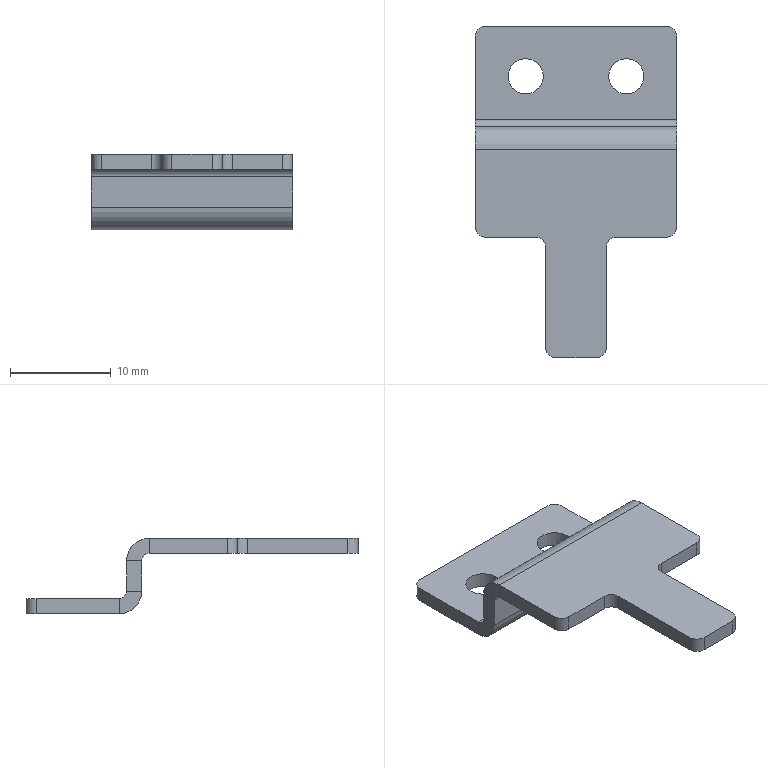Part | STEP file | 10-17 shaft sensor plate (Default) | 1 solid | 38 faces | box 20 x 33 x 7.5 mm | volume 849.566 mm3 | plane 22 | cylinder 16 | commonest cylinder face diameters 2 x8 3.5 x4 1.473 x2 4.473 x2
STEP:
#1=CARTESIAN_POINT('',(-6.75,0.,-1.5));
#2=VERTEX_POINT('',#1);
#3=CARTESIAN_POINT('',(-3.25,0.,-1.5));
#4=VERTEX_POINT('',#3);
#5=CARTESIAN_POINT('',(-5.,0.,-1.5));
#6=DIRECTION('',(0.,0.,1.));
#7=DIRECTION('',(1.,0.,0.));
#8=AXIS2_PLACEMENT_3D('',#5,#6,#7);
#9=CIRCLE('',#8,1.75);
#10=EDGE_CURVE('',#2,#4,#9,.T.);
#11=ORIENTED_EDGE('',*,*,#10,.F.);
#12=CARTESIAN_POINT('',(-6.75,0.,0.));
#13=VERTEX_POINT('',#12);
#14=CARTESIAN_POINT('',(-6.75,0.,0.));
#15=DIRECTION('',(0.,0.,1.));
#16=VECTOR('',#15,1000.);
#17=LINE('',#14,#16);
#18=EDGE_CURVE('',#2,#13,#17,.T.);
#19=ORIENTED_EDGE('',*,*,#18,.T.);
#20=CARTESIAN_POINT('',(-3.25,0.,0.));
#21=VERTEX_POINT('',#20);
#22=CARTESIAN_POINT('',(-5.,0.,0.));
#23=DIRECTION('',(0.,0.,1.));
#24=DIRECTION('',(1.,0.,0.));
#25=AXIS2_PLACEMENT_3D('',#22,#23,#24);
#26=CIRCLE('',#25,1.75);
#27=EDGE_CURVE('',#13,#21,#26,.T.);
#28=ORIENTED_EDGE('',*,*,#27,.T.);
#29=CARTESIAN_POINT('',(-3.25,0.,0.));
#30=DIRECTION('',(0.,0.,1.));
#31=VECTOR('',#30,1000.);
#32=LINE('',#29,#31);
#33=EDGE_CURVE('',#4,#21,#32,.T.);
#34=ORIENTED_EDGE('',*,*,#33,.F.);
#35=EDGE_LOOP('',(#11,#19,#28,#34));
#36=FACE_OUTER_BOUND('',#35,.T.);
#37=CARTESIAN_POINT('',(-5.,0.,0.));
#38=DIRECTION('',(0.,0.,1.));
#39=DIRECTION('',(1.,0.,0.));
#40=AXIS2_PLACEMENT_3D('',#37,#38,#39);
#41=CYLINDRICAL_SURFACE('',#40,1.75);
#42=ADVANCED_FACE('',(#36),#41,.F.);
#43=CARTESIAN_POINT('',(3.25,0.,-1.5));
#44=VERTEX_POINT('',#43);
#45=CARTESIAN_POINT('',(6.75,0.,-1.5));
#46=VERTEX_POINT('',#45);
#47=CARTESIAN_POINT('',(5.,0.,-1.5));
#48=DIRECTION('',(0.,0.,1.));
#49=DIRECTION('',(1.,0.,0.));
#50=AXIS2_PLACEMENT_3D('',#47,#48,#49);
#51=CIRCLE('',#50,1.75);
#52=EDGE_CURVE('',#44,#46,#51,.T.);
#53=ORIENTED_EDGE('',*,*,#52,.F.);
#54=CARTESIAN_POINT('',(3.25,0.,0.));
#55=VERTEX_POINT('',#54);
#56=CARTESIAN_POINT('',(3.25,0.,0.));
#57=DIRECTION('',(0.,0.,1.));
#58=VECTOR('',#57,1000.);
#59=LINE('',#56,#58);
#60=EDGE_CURVE('',#44,#55,#59,.T.);
#61=ORIENTED_EDGE('',*,*,#60,.T.);
#62=CARTESIAN_POINT('',(6.75,0.,0.));
#63=VERTEX_POINT('',#62);
#64=CARTESIAN_POINT('',(5.,0.,0.));
#65=DIRECTION('',(0.,0.,1.));
#66=DIRECTION('',(1.,0.,0.));
#67=AXIS2_PLACEMENT_3D('',#64,#65,#66);
#68=CIRCLE('',#67,1.75);
#69=EDGE_CURVE('',#55,#63,#68,.T.);
#70=ORIENTED_EDGE('',*,*,#69,.T.);
#71=CARTESIAN_POINT('',(6.75,0.,0.));
#72=DIRECTION('',(0.,0.,1.));
#73=VECTOR('',#72,1000.);
#74=LINE('',#71,#73);
#75=EDGE_CURVE('',#46,#63,#74,.T.);
#76=ORIENTED_EDGE('',*,*,#75,.F.);
#77=EDGE_LOOP('',(#53,#61,#70,#76));
#78=FACE_OUTER_BOUND('',#77,.T.);
#79=CARTESIAN_POINT('',(5.,0.,0.));
#80=DIRECTION('',(0.,0.,1.));
#81=DIRECTION('',(1.,0.,0.));
#82=AXIS2_PLACEMENT_3D('',#79,#80,#81);
#83=CYLINDRICAL_SURFACE('',#82,1.75);
#84=ADVANCED_FACE('',(#78),#83,.F.);
#85=CARTESIAN_POINT('',(-10.,-6.5,0.7366));
#86=VERTEX_POINT('',#85);
#87=CARTESIAN_POINT('',(-10.,-6.5,3.763));
#88=VERTEX_POINT('',#87);
#89=CARTESIAN_POINT('',(-10.,-6.5,4.5));
#90=DIRECTION('',(0.,0.,1.));
#91=VECTOR('',#90,1000.);
#92=LINE('',#89,#91);
#93=EDGE_CURVE('',#86,#88,#92,.T.);
#94=ORIENTED_EDGE('',*,*,#93,.T.);
#95=CARTESIAN_POINT('',(-10.,-5.,3.763));
#96=VERTEX_POINT('',#95);
#97=CARTESIAN_POINT('',(-10.,-6.5,3.763));
#98=DIRECTION('',(0.,1.,0.));
#99=VECTOR('',#98,1000.);
#100=LINE('',#97,#99);
#101=EDGE_CURVE('',#88,#96,#100,.T.);
#102=ORIENTED_EDGE('',*,*,#101,.T.);
#103=CARTESIAN_POINT('',(-10.,-5.,0.7366));
#104=VERTEX_POINT('',#103);
#105=CARTESIAN_POINT('',(-10.,-5.,4.5));
#106=DIRECTION('',(0.,0.,1.));
#107=VECTOR('',#106,1000.);
#108=LINE('',#105,#107);
#109=EDGE_CURVE('',#104,#96,#108,.T.);
#110=ORIENTED_EDGE('',*,*,#109,.F.);
#111=CARTESIAN_POINT('',(-10.,-5.,0.7366));
#112=DIRECTION('',(0.,-1.,0.));
#113=VECTOR('',#112,1000.);
#114=LINE('',#111,#113);
#115=EDGE_CURVE('',#104,#86,#114,.T.);
#116=ORIENTED_EDGE('',*,*,#115,.T.);
#117=EDGE_LOOP('',(#94,#102,#110,#116));
#118=FACE_OUTER_BOUND('',#117,.T.);
#119=CARTESIAN_POINT('',(-10.,-6.5,4.5));
#120=DIRECTION('',(-1.,0.,0.));
#121=DIRECTION('',(0.,0.,1.));
#122=AXIS2_PLACEMENT_3D('',#119,#120,#121);
#123=PLANE('',#122);
#124=ADVANCED_FACE('',(#118),#123,.T.);
#125=CARTESIAN_POINT('',(10.,-6.5,3.763));
#126=VERTEX_POINT('',#125);
#127=CARTESIAN_POINT('',(10.,-6.5,0.7366));
#128=VERTEX_POINT('',#127);
#129=CARTESIAN_POINT('',(10.,-6.5,0.));
#130=DIRECTION('',(0.,0.,-1.));
#131=VECTOR('',#130,1000.);
#132=LINE('',#129,#131);
#133=EDGE_CURVE('',#126,#128,#132,.T.);
#134=ORIENTED_EDGE('',*,*,#133,.F.);
#135=CARTESIAN_POINT('',(-10.,-6.5,3.763));
#136=DIRECTION('',(1.,0.,0.));
#137=VECTOR('',#136,1000.);
#138=LINE('',#135,#137);
#139=EDGE_CURVE('',#88,#126,#138,.T.);
#140=ORIENTED_EDGE('',*,*,#139,.F.);
#141=ORIENTED_EDGE('',*,*,#93,.F.);
#142=CARTESIAN_POINT('',(10.,-6.5,0.7366));
#143=DIRECTION('',(1.,0.,0.));
#144=VECTOR('',#143,1000.);
#145=LINE('',#142,#144);
#146=EDGE_CURVE('',#86,#128,#145,.T.);
#147=ORIENTED_EDGE('',*,*,#146,.T.);
#148=EDGE_LOOP('',(#134,#140,#141,#147));
#149=FACE_OUTER_BOUND('',#148,.T.);
#150=CARTESIAN_POINT('',(10.,-6.5,0.));
#151=DIRECTION('',(0.,-1.,0.));
#152=DIRECTION('',(0.,0.,-1.));
#153=AXIS2_PLACEMENT_3D('',#150,#151,#152);
#154=PLANE('',#153);
#155=ADVANCED_FACE('',(#149),#154,.T.);
#156=CARTESIAN_POINT('',(10.,-5.,3.763));
#157=VERTEX_POINT('',#156);
#158=CARTESIAN_POINT('',(-10.,-5.,3.763));
#159=DIRECTION('',(1.,0.,0.));
#160=VECTOR('',#159,1000.);
#161=LINE('',#158,#160);
#162=EDGE_CURVE('',#96,#157,#161,.T.);
#163=ORIENTED_EDGE('',*,*,#162,.T.);
#164=CARTESIAN_POINT('',(10.,-5.,0.7366));
#165=VERTEX_POINT('',#164);
#166=CARTESIAN_POINT('',(10.,-5.,0.));
#167=DIRECTION('',(0.,0.,-1.));
#168=VECTOR('',#167,1000.);
#169=LINE('',#166,#168);
#170=EDGE_CURVE('',#157,#165,#169,.T.);
#171=ORIENTED_EDGE('',*,*,#170,.T.);
#172=CARTESIAN_POINT('',(-10.,-5.,0.7366));
#173=DIRECTION('',(1.,0.,0.));
#174=VECTOR('',#173,1000.);
#175=LINE('',#172,#174);
#176=EDGE_CURVE('',#104,#165,#175,.T.);
#177=ORIENTED_EDGE('',*,*,#176,.F.);
#178=ORIENTED_EDGE('',*,*,#109,.T.);
#179=EDGE_LOOP('',(#163,#171,#177,#178));
#180=FACE_OUTER_BOUND('',#179,.T.);
#181=CARTESIAN_POINT('',(10.,-5.,0.));
#182=DIRECTION('',(0.,-1.,0.));
#183=DIRECTION('',(0.,0.,-1.));
#184=AXIS2_PLACEMENT_3D('',#181,#182,#183);
#185=PLANE('',#184);
#186=ADVANCED_FACE('',(#180),#185,.F.);
#187=CARTESIAN_POINT('',(10.,-4.263,-1.5));
#188=VERTEX_POINT('',#187);
#189=CARTESIAN_POINT('',(10.,4.,-1.5));
#190=VERTEX_POINT('',#189);
#191=CARTESIAN_POINT('',(10.,5.,-1.5));
#192=DIRECTION('',(0.,1.,0.));
#193=VECTOR('',#192,1000.);
#194=LINE('',#191,#193);
#195=EDGE_CURVE('',#188,#190,#194,.T.);
#196=ORIENTED_EDGE('',*,*,#195,.T.);
#197=CARTESIAN_POINT('',(10.,4.,0.));
#198=VERTEX_POINT('',#197);
#199=CARTESIAN_POINT('',(10.,4.,-1.5));
#200=DIRECTION('',(0.,0.,1.));
#201=VECTOR('',#200,1000.);
#202=LINE('',#199,#201);
#203=EDGE_CURVE('',#190,#198,#202,.T.);
#204=ORIENTED_EDGE('',*,*,#203,.T.);
#205=CARTESIAN_POINT('',(10.,-4.263,0.));
#206=VERTEX_POINT('',#205);
#207=CARTESIAN_POINT('',(10.,5.,0.));
#208=DIRECTION('',(0.,1.,0.));
#209=VECTOR('',#208,1000.);
#210=LINE('',#207,#209);
#211=EDGE_CURVE('',#206,#198,#210,.T.);
#212=ORIENTED_EDGE('',*,*,#211,.F.);
#213=CARTESIAN_POINT('',(10.,-4.263,0.));
#214=DIRECTION('',(0.,0.,-1.));
#215=VECTOR('',#214,1000.);
#216=LINE('',#213,#215);
#217=EDGE_CURVE('',#206,#188,#216,.T.);
#218=ORIENTED_EDGE('',*,*,#217,.T.);
#219=EDGE_LOOP('',(#196,#204,#212,#218));
#220=FACE_OUTER_BOUND('',#219,.T.);
#221=CARTESIAN_POINT('',(10.,5.,-1.5));
#222=DIRECTION('',(1.,0.,0.));
#223=DIRECTION('',(0.,1.,0.));
#224=AXIS2_PLACEMENT_3D('',#221,#222,#223);
#225=PLANE('',#224);
#226=ADVANCED_FACE('',(#220),#225,.T.);
#227=CARTESIAN_POINT('',(5.,0.,-1.5));
#228=DIRECTION('',(0.,0.,1.));
#229=DIRECTION('',(1.,0.,0.));
#230=AXIS2_PLACEMENT_3D('',#227,#228,#229);
#231=CIRCLE('',#230,1.75);
#232=EDGE_CURVE('',#46,#44,#231,.T.);
#233=ORIENTED_EDGE('',*,*,#232,.T.);
#234=ORIENTED_EDGE('',*,*,#52,.T.);
#235=EDGE_LOOP('',(#233,#234));
#236=FACE_BOUND('',#235,.T.);
#237=CARTESIAN_POINT('',(-5.,0.,-1.5));
#238=DIRECTION('',(0.,0.,1.));
#239=DIRECTION('',(1.,0.,0.));
#240=AXIS2_PLACEMENT_3D('',#237,#238,#239);
#241=CIRCLE('',#240,1.75);
#242=EDGE_CURVE('',#4,#2,#241,.T.);
#243=ORIENTED_EDGE('',*,*,#242,.T.);
#244=ORIENTED_EDGE('',*,*,#10,.T.);
#245=EDGE_LOOP('',(#243,#244));
#246=FACE_BOUND('',#245,.T.);
#247=CARTESIAN_POINT('',(-10.,4.,-1.5));
#248=VERTEX_POINT('',#247);
#249=CARTESIAN_POINT('',(-10.,-4.263,-1.5));
#250=VERTEX_POINT('',#249);
#251=CARTESIAN_POINT('',(-10.,5.,-1.5));
#252=DIRECTION('',(0.,-1.,0.));
#253=VECTOR('',#252,1000.);
#254=LINE('',#251,#253);
#255=EDGE_CURVE('',#248,#250,#254,.T.);
#256=ORIENTED_EDGE('',*,*,#255,.F.);
#257=CARTESIAN_POINT('',(-9.,5.,-1.5));
#258=VERTEX_POINT('',#257);
#259=CARTESIAN_POINT('',(-9.,4.,-1.5));
#260=DIRECTION('',(0.,0.,-1.));
#261=DIRECTION('',(1.,0.,0.));
#262=AXIS2_PLACEMENT_3D('',#259,#260,#261);
#263=CIRCLE('',#262,1.);
#264=EDGE_CURVE('',#248,#258,#263,.T.);
#265=ORIENTED_EDGE('',*,*,#264,.T.);
#266=CARTESIAN_POINT('',(9.,5.,-1.5));
#267=VERTEX_POINT('',#266);
#268=CARTESIAN_POINT('',(-10.,5.,-1.5));
#269=DIRECTION('',(-1.,0.,0.));
#270=VECTOR('',#269,1000.);
#271=LINE('',#268,#270);
#272=EDGE_CURVE('',#267,#258,#271,.T.);
#273=ORIENTED_EDGE('',*,*,#272,.F.);
#274=CARTESIAN_POINT('',(9.,4.,-1.5));
#275=DIRECTION('',(0.,0.,-1.));
#276=DIRECTION('',(1.,0.,0.));
#277=AXIS2_PLACEMENT_3D('',#274,#275,#276);
#278=CIRCLE('',#277,1.);
#279=EDGE_CURVE('',#267,#190,#278,.T.);
#280=ORIENTED_EDGE('',*,*,#279,.T.);
#281=ORIENTED_EDGE('',*,*,#195,.F.);
#282=CARTESIAN_POINT('',(10.,-4.263,-1.5));
#283=DIRECTION('',(-1.,0.,0.));
#284=VECTOR('',#283,1000.);
#285=LINE('',#282,#284);
#286=EDGE_CURVE('',#188,#250,#285,.T.);
#287=ORIENTED_EDGE('',*,*,#286,.T.);
#288=EDGE_LOOP('',(#256,#265,#273,#280,#281,#287));
#289=FACE_OUTER_BOUND('',#288,.T.);
#290=CARTESIAN_POINT('',(10.,-5.,-1.5));
#291=DIRECTION('',(0.,0.,1.));
#292=DIRECTION('',(1.,0.,0.));
#293=AXIS2_PLACEMENT_3D('',#290,#291,#292);
#294=PLANE('',#293);
#295=ADVANCED_FACE('',(#236,#246,#289),#294,.F.);
#296=CARTESIAN_POINT('',(5.,0.,0.));
#297=DIRECTION('',(0.,0.,1.));
#298=DIRECTION('',(1.,0.,0.));
#299=AXIS2_PLACEMENT_3D('',#296,#297,#298);
#300=CIRCLE('',#299,1.75);
#301=EDGE_CURVE('',#63,#55,#300,.T.);
#302=ORIENTED_EDGE('',*,*,#301,.F.);
#303=ORIENTED_EDGE('',*,*,#69,.F.);
#304=EDGE_LOOP('',(#302,#303));
#305=FACE_BOUND('',#304,.T.);
#306=CARTESIAN_POINT('',(-5.,0.,0.));
#307=DIRECTION('',(0.,0.,1.));
#308=DIRECTION('',(1.,0.,0.));
#309=AXIS2_PLACEMENT_3D('',#306,#307,#308);
#310=CIRCLE('',#309,1.75);
#311=EDGE_CURVE('',#21,#13,#310,.T.);
#312=ORIENTED_EDGE('',*,*,#311,.F.);
#313=ORIENTED_EDGE('',*,*,#27,.F.);
#314=EDGE_LOOP('',(#312,#313));
#315=FACE_BOUND('',#314,.T.);
#316=CARTESIAN_POINT('',(9.,5.,0.));
#317=VERTEX_POINT('',#316);
#318=CARTESIAN_POINT('',(-9.,5.,0.));
#319=VERTEX_POINT('',#318);
#320=CARTESIAN_POINT('',(-10.,5.,0.));
#321=DIRECTION('',(-1.,0.,0.));
#322=VECTOR('',#321,1000.);
#323=LINE('',#320,#322);
#324=EDGE_CURVE('',#317,#319,#323,.T.);
#325=ORIENTED_EDGE('',*,*,#324,.T.);
#326=CARTESIAN_POINT('',(-10.,4.,0.));
#327=VERTEX_POINT('',#326);
#328=CARTESIAN_POINT('',(-9.,4.,0.));
#329=DIRECTION('',(0.,0.,1.));
#330=DIRECTION('',(1.,0.,0.));
#331=AXIS2_PLACEMENT_3D('',#328,#329,#330);
#332=CIRCLE('',#331,1.);
#333=EDGE_CURVE('',#319,#327,#332,.T.);
#334=ORIENTED_EDGE('',*,*,#333,.T.);
#335=CARTESIAN_POINT('',(-10.,-4.263,0.));
#336=VERTEX_POINT('',#335);
#337=CARTESIAN_POINT('',(-10.,5.,0.));
#338=DIRECTION('',(0.,-1.,0.));
#339=VECTOR('',#338,1000.);
#340=LINE('',#337,#339);
#341=EDGE_CURVE('',#327,#336,#340,.T.);
#342=ORIENTED_EDGE('',*,*,#341,.T.);
#343=CARTESIAN_POINT('',(10.,-4.263,0.));
#344=DIRECTION('',(-1.,0.,0.));
#345=VECTOR('',#344,1000.);
#346=LINE('',#343,#345);
#347=EDGE_CURVE('',#206,#336,#346,.T.);
#348=ORIENTED_EDGE('',*,*,#347,.F.);
#349=ORIENTED_EDGE('',*,*,#211,.T.);
#350=CARTESIAN_POINT('',(9.,4.,0.));
#351=DIRECTION('',(0.,0.,1.));
#352=DIRECTION('',(1.,0.,0.));
#353=AXIS2_PLACEMENT_3D('',#350,#351,#352);
#354=CIRCLE('',#353,1.);
#355=EDGE_CURVE('',#198,#317,#354,.T.);
#356=ORIENTED_EDGE('',*,*,#355,.T.);
#357=EDGE_LOOP('',(#325,#334,#342,#348,#349,#356));
#358=FACE_OUTER_BOUND('',#357,.T.);
#359=CARTESIAN_POINT('',(10.,-5.,0.));
#360=DIRECTION('',(0.,0.,1.));
#361=DIRECTION('',(1.,0.,0.));
#362=AXIS2_PLACEMENT_3D('',#359,#360,#361);
#363=PLANE('',#362);
#364=ADVANCED_FACE('',(#305,#315,#358),#363,.T.);
#365=ORIENTED_EDGE('',*,*,#341,.F.);
#366=CARTESIAN_POINT('',(-10.,4.,-1.5));
#367=DIRECTION('',(0.,0.,-1.));
#368=VECTOR('',#367,1000.);
#369=LINE('',#366,#368);
#370=EDGE_CURVE('',#327,#248,#369,.T.);
#371=ORIENTED_EDGE('',*,*,#370,.T.);
#372=ORIENTED_EDGE('',*,*,#255,.T.);
#373=CARTESIAN_POINT('',(-10.,-4.263,0.));
#374=DIRECTION('',(0.,0.,-1.));
#375=VECTOR('',#374,1000.);
#376=LINE('',#373,#375);
#377=EDGE_CURVE('',#336,#250,#376,.T.);
#378=ORIENTED_EDGE('',*,*,#377,.F.);
#379=EDGE_LOOP('',(#365,#371,#372,#378));
#380=FACE_OUTER_BOUND('',#379,.T.);
#381=CARTESIAN_POINT('',(-10.,5.,-1.5));
#382=DIRECTION('',(-1.,0.,0.));
#383=DIRECTION('',(0.,-1.,0.));
#384=AXIS2_PLACEMENT_3D('',#381,#382,#383);
#385=PLANE('',#384);
#386=ADVANCED_FACE('',(#380),#385,.T.);
#387=ORIENTED_EDGE('',*,*,#272,.T.);
#388=CARTESIAN_POINT('',(-9.,5.,-1.5));
#389=DIRECTION('',(0.,0.,1.));
#390=VECTOR('',#389,1000.);
#391=LINE('',#388,#390);
#392=EDGE_CURVE('',#258,#319,#391,.T.);
#393=ORIENTED_EDGE('',*,*,#392,.T.);
#394=ORIENTED_EDGE('',*,*,#324,.F.);
#395=CARTESIAN_POINT('',(9.,5.,-1.5));
#396=DIRECTION('',(0.,0.,-1.));
#397=VECTOR('',#396,1000.);
#398=LINE('',#395,#397);
#399=EDGE_CURVE('',#317,#267,#398,.T.);
#400=ORIENTED_EDGE('',*,*,#399,.T.);
#401=EDGE_LOOP('',(#387,#393,#394,#400));
#402=FACE_OUTER_BOUND('',#401,.T.);
#403=CARTESIAN_POINT('',(-10.,5.,-1.5));
#404=DIRECTION('',(0.,1.,0.));
#405=DIRECTION('',(0.,0.,1.));
#406=AXIS2_PLACEMENT_3D('',#403,#404,#405);
#407=PLANE('',#406);
#408=ADVANCED_FACE('',(#402),#407,.T.);
#409=ORIENTED_EDGE('',*,*,#60,.F.);
#410=ORIENTED_EDGE('',*,*,#232,.F.);
#411=ORIENTED_EDGE('',*,*,#75,.T.);
#412=ORIENTED_EDGE('',*,*,#301,.T.);
#413=EDGE_LOOP('',(#409,#410,#411,#412));
#414=FACE_OUTER_BOUND('',#413,.T.);
#415=CARTESIAN_POINT('',(5.,0.,0.));
#416=DIRECTION('',(0.,0.,1.));
#417=DIRECTION('',(1.,0.,0.));
#418=AXIS2_PLACEMENT_3D('',#415,#416,#417);
#419=CYLINDRICAL_SURFACE('',#418,1.75);
#420=ADVANCED_FACE('',(#414),#419,.F.);
#421=ORIENTED_EDGE('',*,*,#18,.F.);
#422=ORIENTED_EDGE('',*,*,#242,.F.);
#423=ORIENTED_EDGE('',*,*,#33,.T.);
#424=ORIENTED_EDGE('',*,*,#311,.T.);
#425=EDGE_LOOP('',(#421,#422,#423,#424));
#426=FACE_OUTER_BOUND('',#425,.T.);
#427=CARTESIAN_POINT('',(-5.,0.,0.));
#428=DIRECTION('',(0.,0.,1.));
#429=DIRECTION('',(1.,0.,0.));
#430=AXIS2_PLACEMENT_3D('',#427,#428,#429);
#431=CYLINDRICAL_SURFACE('',#430,1.75);
#432=ADVANCED_FACE('',(#426),#431,.F.);
#433=ORIENTED_EDGE('',*,*,#115,.F.);
#434=CARTESIAN_POINT('',(-10.,-4.263,0.7366));
#435=DIRECTION('',(-1.,0.,0.));
#436=DIRECTION('',(0.,0.,-1.));
#437=AXIS2_PLACEMENT_3D('',#434,#435,#436);
#438=CIRCLE('',#437,0.7366);
#439=EDGE_CURVE('',#336,#104,#438,.T.);
#440=ORIENTED_EDGE('',*,*,#439,.F.);
#441=ORIENTED_EDGE('',*,*,#377,.T.);
#442=CARTESIAN_POINT('',(-10.,-4.263,0.7366));
#443=DIRECTION('',(-1.,0.,0.));
#444=DIRECTION('',(0.,0.,-1.));
#445=AXIS2_PLACEMENT_3D('',#442,#443,#444);
#446=CIRCLE('',#445,2.237);
#447=EDGE_CURVE('',#250,#86,#446,.T.);
#448=ORIENTED_EDGE('',*,*,#447,.T.);
#449=EDGE_LOOP('',(#433,#440,#441,#448));
#450=FACE_OUTER_BOUND('',#449,.T.);
#451=CARTESIAN_POINT('',(-10.,-4.263,0.7366));
#452=DIRECTION('',(-1.,0.,0.));
#453=DIRECTION('',(0.,0.,1.));
#454=AXIS2_PLACEMENT_3D('',#451,#452,#453);
#455=PLANE('',#454);
#456=ADVANCED_FACE('',(#450),#455,.T.);
#457=CARTESIAN_POINT('',(10.,-4.263,0.7366));
#458=DIRECTION('',(1.,0.,0.));
#459=DIRECTION('',(0.,0.,-1.));
#460=AXIS2_PLACEMENT_3D('',#457,#458,#459);
#461=CIRCLE('',#460,0.7366);
#462=EDGE_CURVE('',#165,#206,#461,.T.);
#463=ORIENTED_EDGE('',*,*,#462,.F.);
#464=CARTESIAN_POINT('',(10.,-5.,0.7366));
#465=DIRECTION('',(0.,-1.,0.));
#466=VECTOR('',#465,1000.);
#467=LINE('',#464,#466);
#468=EDGE_CURVE('',#165,#128,#467,.T.);
#469=ORIENTED_EDGE('',*,*,#468,.T.);
#470=CARTESIAN_POINT('',(10.,-4.263,0.7366));
#471=DIRECTION('',(1.,0.,0.));
#472=DIRECTION('',(0.,0.,-1.));
#473=AXIS2_PLACEMENT_3D('',#470,#471,#472);
#474=CIRCLE('',#473,2.237);
#475=EDGE_CURVE('',#128,#188,#474,.T.);
#476=ORIENTED_EDGE('',*,*,#475,.T.);
#477=ORIENTED_EDGE('',*,*,#217,.F.);
#478=EDGE_LOOP('',(#463,#469,#476,#477));
#479=FACE_OUTER_BOUND('',#478,.T.);
#480=CARTESIAN_POINT('',(10.,-4.263,0.7366));
#481=DIRECTION('',(-1.,0.,0.));
#482=DIRECTION('',(0.,0.,1.));
#483=AXIS2_PLACEMENT_3D('',#480,#481,#482);
#484=PLANE('',#483);
#485=ADVANCED_FACE('',(#479),#484,.F.);
#486=ORIENTED_EDGE('',*,*,#286,.F.);
#487=ORIENTED_EDGE('',*,*,#475,.F.);
#488=ORIENTED_EDGE('',*,*,#146,.F.);
#489=ORIENTED_EDGE('',*,*,#447,.F.);
#490=EDGE_LOOP('',(#486,#487,#488,#489));
#491=FACE_OUTER_BOUND('',#490,.T.);
#492=CARTESIAN_POINT('',(10.,-4.263,0.7366));
#493=DIRECTION('',(1.,0.,0.));
#494=DIRECTION('',(0.,-1.,0.));
#495=AXIS2_PLACEMENT_3D('',#492,#493,#494);
#496=CYLINDRICAL_SURFACE('',#495,2.237);
#497=ADVANCED_FACE('',(#491),#496,.T.);
#498=ORIENTED_EDGE('',*,*,#347,.T.);
#499=ORIENTED_EDGE('',*,*,#439,.T.);
#500=ORIENTED_EDGE('',*,*,#176,.T.);
#501=ORIENTED_EDGE('',*,*,#462,.T.);
#502=EDGE_LOOP('',(#498,#499,#500,#501));
#503=FACE_OUTER_BOUND('',#502,.T.);
#504=CARTESIAN_POINT('',(10.,-4.263,0.7366));
#505=DIRECTION('',(1.,0.,0.));
#506=DIRECTION('',(0.,-1.,0.));
#507=AXIS2_PLACEMENT_3D('',#504,#505,#506);
#508=CYLINDRICAL_SURFACE('',#507,0.7366);
#509=ADVANCED_FACE('',(#503),#508,.F.);
#510=CARTESIAN_POINT('',(10.,-6.5,3.763));
#511=DIRECTION('',(0.,1.,0.));
#512=VECTOR('',#511,1000.);
#513=LINE('',#510,#512);
#514=EDGE_CURVE('',#126,#157,#513,.T.);
#515=ORIENTED_EDGE('',*,*,#514,.F.);
#516=ORIENTED_EDGE('',*,*,#133,.T.);
#517=ORIENTED_EDGE('',*,*,#468,.F.);
#518=ORIENTED_EDGE('',*,*,#170,.F.);
#519=EDGE_LOOP('',(#515,#516,#517,#518));
#520=FACE_OUTER_BOUND('',#519,.T.);
#521=CARTESIAN_POINT('',(10.,-6.5,0.));
#522=DIRECTION('',(1.,0.,0.));
#523=DIRECTION('',(0.,0.,-1.));
#524=AXIS2_PLACEMENT_3D('',#521,#522,#523);
#525=PLANE('',#524);
#526=ADVANCED_FACE('',(#520),#525,.T.);
#527=CARTESIAN_POINT('',(10.,-7.237,4.5));
#528=VERTEX_POINT('',#527);
#529=CARTESIAN_POINT('',(10.,-7.237,6.));
#530=VERTEX_POINT('',#529);
#531=CARTESIAN_POINT('',(10.,-7.237,4.5));
#532=DIRECTION('',(0.,0.,1.));
#533=VECTOR('',#532,1000.);
#534=LINE('',#531,#533);
#535=EDGE_CURVE('',#528,#530,#534,.T.);
#536=ORIENTED_EDGE('',*,*,#535,.F.);
#537=CARTESIAN_POINT('',(10.,-7.237,3.763));
#538=DIRECTION('',(1.,0.,0.));
#539=DIRECTION('',(0.,0.,1.));
#540=AXIS2_PLACEMENT_3D('',#537,#538,#539);
#541=CIRCLE('',#540,0.7366);
#542=EDGE_CURVE('',#126,#528,#541,.T.);
#543=ORIENTED_EDGE('',*,*,#542,.F.);
#544=ORIENTED_EDGE('',*,*,#514,.T.);
#545=CARTESIAN_POINT('',(10.,-7.237,3.763));
#546=DIRECTION('',(1.,0.,0.));
#547=DIRECTION('',(0.,0.,1.));
#548=AXIS2_PLACEMENT_3D('',#545,#546,#547);
#549=CIRCLE('',#548,2.237);
#550=EDGE_CURVE('',#157,#530,#549,.T.);
#551=ORIENTED_EDGE('',*,*,#550,.T.);
#552=EDGE_LOOP('',(#536,#543,#544,#551));
#553=FACE_OUTER_BOUND('',#552,.T.);
#554=CARTESIAN_POINT('',(10.,-7.237,3.763));
#555=DIRECTION('',(1.,0.,0.));
#556=DIRECTION('',(0.,0.,-1.));
#557=AXIS2_PLACEMENT_3D('',#554,#555,#556);
#558=PLANE('',#557);
#559=ADVANCED_FACE('',(#553),#558,.T.);
#560=CARTESIAN_POINT('',(-10.,-7.237,4.5));
#561=VERTEX_POINT('',#560);
#562=CARTESIAN_POINT('',(-10.,-7.237,3.763));
#563=DIRECTION('',(-1.,0.,0.));
#564=DIRECTION('',(0.,0.,1.));
#565=AXIS2_PLACEMENT_3D('',#562,#563,#564);
#566=CIRCLE('',#565,0.7366);
#567=EDGE_CURVE('',#561,#88,#566,.T.);
#568=ORIENTED_EDGE('',*,*,#567,.F.);
#569=CARTESIAN_POINT('',(-10.,-7.237,6.));
#570=VERTEX_POINT('',#569);
#571=CARTESIAN_POINT('',(-10.,-7.237,4.5));
#572=DIRECTION('',(0.,0.,1.));
#573=VECTOR('',#572,1000.);
#574=LINE('',#571,#573);
#575=EDGE_CURVE('',#561,#570,#574,.T.);
#576=ORIENTED_EDGE('',*,*,#575,.T.);
#577=CARTESIAN_POINT('',(-10.,-7.237,3.763));
#578=DIRECTION('',(-1.,0.,0.));
#579=DIRECTION('',(0.,0.,1.));
#580=AXIS2_PLACEMENT_3D('',#577,#578,#579);
#581=CIRCLE('',#580,2.237);
#582=EDGE_CURVE('',#570,#96,#581,.T.);
#583=ORIENTED_EDGE('',*,*,#582,.T.);
#584=ORIENTED_EDGE('',*,*,#101,.F.);
#585=EDGE_LOOP('',(#568,#576,#583,#584));
#586=FACE_OUTER_BOUND('',#585,.T.);
#587=CARTESIAN_POINT('',(-10.,-7.237,3.763));
#588=DIRECTION('',(1.,0.,0.));
#589=DIRECTION('',(0.,0.,-1.));
#590=AXIS2_PLACEMENT_3D('',#587,#588,#589);
#591=PLANE('',#590);
#592=ADVANCED_FACE('',(#586),#591,.F.);
#593=ORIENTED_EDGE('',*,*,#162,.F.);
#594=ORIENTED_EDGE('',*,*,#582,.F.);
#595=CARTESIAN_POINT('',(-10.,-7.237,6.));
#596=DIRECTION('',(-1.,0.,0.));
#597=VECTOR('',#596,1000.);
#598=LINE('',#595,#597);
#599=EDGE_CURVE('',#530,#570,#598,.T.);
#600=ORIENTED_EDGE('',*,*,#599,.F.);
#601=ORIENTED_EDGE('',*,*,#550,.F.);
#602=EDGE_LOOP('',(#593,#594,#600,#601));
#603=FACE_OUTER_BOUND('',#602,.T.);
#604=CARTESIAN_POINT('',(-10.,-7.237,3.763));
#605=DIRECTION('',(-1.,0.,0.));
#606=DIRECTION('',(0.,0.,1.));
#607=AXIS2_PLACEMENT_3D('',#604,#605,#606);
#608=CYLINDRICAL_SURFACE('',#607,2.237);
#609=ADVANCED_FACE('',(#603),#608,.T.);
#610=ORIENTED_EDGE('',*,*,#139,.T.);
#611=ORIENTED_EDGE('',*,*,#542,.T.);
#612=CARTESIAN_POINT('',(10.,-7.237,4.5));
#613=DIRECTION('',(-1.,0.,0.));
#614=VECTOR('',#613,1000.);
#615=LINE('',#612,#614);
#616=EDGE_CURVE('',#528,#561,#615,.T.);
#617=ORIENTED_EDGE('',*,*,#616,.T.);
#618=ORIENTED_EDGE('',*,*,#567,.T.);
#619=EDGE_LOOP('',(#610,#611,#617,#618));
#620=FACE_OUTER_BOUND('',#619,.T.);
#621=CARTESIAN_POINT('',(-10.,-7.237,3.763));
#622=DIRECTION('',(-1.,0.,0.));
#623=DIRECTION('',(0.,0.,1.));
#624=AXIS2_PLACEMENT_3D('',#621,#622,#623);
#625=CYLINDRICAL_SURFACE('',#624,0.7366);
#626=ADVANCED_FACE('',(#620),#625,.F.);
#627=CARTESIAN_POINT('',(-10.,-15.,4.5));
#628=VERTEX_POINT('',#627);
#629=CARTESIAN_POINT('',(-10.,-6.5,4.5));
#630=DIRECTION('',(0.,1.,0.));
#631=VECTOR('',#630,1000.);
#632=LINE('',#629,#631);
#633=EDGE_CURVE('',#628,#561,#632,.T.);
#634=ORIENTED_EDGE('',*,*,#633,.F.);
#635=CARTESIAN_POINT('',(-10.,-15.,6.));
#636=VERTEX_POINT('',#635);
#637=CARTESIAN_POINT('',(-10.,-15.,6.));
#638=DIRECTION('',(0.,0.,1.));
#639=VECTOR('',#638,1000.);
#640=LINE('',#637,#639);
#641=EDGE_CURVE('',#628,#636,#640,.T.);
#642=ORIENTED_EDGE('',*,*,#641,.T.);
#643=CARTESIAN_POINT('',(-10.,-6.5,6.));
#644=DIRECTION('',(0.,1.,0.));
#645=VECTOR('',#644,1000.);
#646=LINE('',#643,#645);
#647=EDGE_CURVE('',#636,#570,#646,.T.);
#648=ORIENTED_EDGE('',*,*,#647,.T.);
#649=ORIENTED_EDGE('',*,*,#575,.F.);
#650=EDGE_LOOP('',(#634,#642,#648,#649));
#651=FACE_OUTER_BOUND('',#650,.T.);
#652=CARTESIAN_POINT('',(-10.,-6.5,6.));
#653=DIRECTION('',(-1.,0.,0.));
#654=DIRECTION('',(0.,0.,1.));
#655=AXIS2_PLACEMENT_3D('',#652,#653,#654);
#656=PLANE('',#655);
#657=ADVANCED_FACE('',(#651),#656,.T.);
#658=CARTESIAN_POINT('',(10.,-15.,6.));
#659=VERTEX_POINT('',#658);
#660=CARTESIAN_POINT('',(10.,-28.,6.));
#661=DIRECTION('',(0.,-1.,0.));
#662=VECTOR('',#661,1000.);
#663=LINE('',#660,#662);
#664=EDGE_CURVE('',#530,#659,#663,.T.);
#665=ORIENTED_EDGE('',*,*,#664,.T.);
#666=CARTESIAN_POINT('',(10.,-15.,4.5));
#667=VERTEX_POINT('',#666);
#668=CARTESIAN_POINT('',(10.,-15.,4.5));
#669=DIRECTION('',(0.,0.,-1.));
#670=VECTOR('',#669,1000.);
#671=LINE('',#668,#670);
#672=EDGE_CURVE('',#659,#667,#671,.T.);
#673=ORIENTED_EDGE('',*,*,#672,.T.);
#674=CARTESIAN_POINT('',(10.,-28.,4.5));
#675=DIRECTION('',(0.,-1.,0.));
#676=VECTOR('',#675,1000.);
#677=LINE('',#674,#676);
#678=EDGE_CURVE('',#528,#667,#677,.T.);
#679=ORIENTED_EDGE('',*,*,#678,.F.);
#680=ORIENTED_EDGE('',*,*,#535,.T.);
#681=EDGE_LOOP('',(#665,#673,#679,#680));
#682=FACE_OUTER_BOUND('',#681,.T.);
#683=CARTESIAN_POINT('',(10.,-28.,6.));
#684=DIRECTION('',(1.,0.,0.));
#685=DIRECTION('',(0.,0.,-1.));
#686=AXIS2_PLACEMENT_3D('',#683,#684,#685);
#687=PLANE('',#686);
#688=ADVANCED_FACE('',(#682),#687,.T.);
#689=ORIENTED_EDGE('',*,*,#647,.F.);
#690=CARTESIAN_POINT('',(-9.,-16.,6.));
#691=VERTEX_POINT('',#690);
#692=CARTESIAN_POINT('',(-9.,-15.,6.));
#693=DIRECTION('',(0.,0.,1.));
#694=DIRECTION('',(0.,-1.,0.));
#695=AXIS2_PLACEMENT_3D('',#692,#693,#694);
#696=CIRCLE('',#695,1.);
#697=EDGE_CURVE('',#636,#691,#696,.T.);
#698=ORIENTED_EDGE('',*,*,#697,.T.);
#699=CARTESIAN_POINT('',(-4.,-16.,6.));
#700=VERTEX_POINT('',#699);
#701=CARTESIAN_POINT('',(-10.,-16.,6.));
#702=DIRECTION('',(-1.,0.,0.));
#703=VECTOR('',#702,1000.);
#704=LINE('',#701,#703);
#705=EDGE_CURVE('',#700,#691,#704,.T.);
#706=ORIENTED_EDGE('',*,*,#705,.F.);
#707=CARTESIAN_POINT('',(-3.,-17.,6.));
#708=VERTEX_POINT('',#707);
#709=CARTESIAN_POINT('',(-4.,-17.,6.));
#710=DIRECTION('',(0.,0.,-1.));
#711=DIRECTION('',(0.,-1.,0.));
#712=AXIS2_PLACEMENT_3D('',#709,#710,#711);
#713=CIRCLE('',#712,1.);
#714=EDGE_CURVE('',#700,#708,#713,.T.);
#715=ORIENTED_EDGE('',*,*,#714,.T.);
#716=CARTESIAN_POINT('',(-3.,-27.,6.));
#717=VERTEX_POINT('',#716);
#718=CARTESIAN_POINT('',(-3.,-28.,6.));
#719=DIRECTION('',(0.,1.,0.));
#720=VECTOR('',#719,1000.);
#721=LINE('',#718,#720);
#722=EDGE_CURVE('',#717,#708,#721,.T.);
#723=ORIENTED_EDGE('',*,*,#722,.F.);
#724=CARTESIAN_POINT('',(-2.,-28.,6.));
#725=VERTEX_POINT('',#724);
#726=CARTESIAN_POINT('',(-2.,-27.,6.));
#727=DIRECTION('',(0.,0.,1.));
#728=DIRECTION('',(0.,-1.,0.));
#729=AXIS2_PLACEMENT_3D('',#726,#727,#728);
#730=CIRCLE('',#729,1.);
#731=EDGE_CURVE('',#717,#725,#730,.T.);
#732=ORIENTED_EDGE('',*,*,#731,.T.);
#733=CARTESIAN_POINT('',(2.,-28.,6.));
#734=VERTEX_POINT('',#733);
#735=CARTESIAN_POINT('',(-10.,-28.,6.));
#736=DIRECTION('',(-1.,0.,0.));
#737=VECTOR('',#736,1000.);
#738=LINE('',#735,#737);
#739=EDGE_CURVE('',#734,#725,#738,.T.);
#740=ORIENTED_EDGE('',*,*,#739,.F.);
#741=CARTESIAN_POINT('',(3.,-27.,6.));
#742=VERTEX_POINT('',#741);
#743=CARTESIAN_POINT('',(2.,-27.,6.));
#744=DIRECTION('',(0.,0.,1.));
#745=DIRECTION('',(0.,-1.,0.));
#746=AXIS2_PLACEMENT_3D('',#743,#744,#745);
#747=CIRCLE('',#746,1.);
#748=EDGE_CURVE('',#734,#742,#747,.T.);
#749=ORIENTED_EDGE('',*,*,#748,.T.);
#750=CARTESIAN_POINT('',(3.,-17.,6.));
#751=VERTEX_POINT('',#750);
#752=CARTESIAN_POINT('',(3.,-28.,6.));
#753=DIRECTION('',(0.,-1.,0.));
#754=VECTOR('',#753,1000.);
#755=LINE('',#752,#754);
#756=EDGE_CURVE('',#751,#742,#755,.T.);
#757=ORIENTED_EDGE('',*,*,#756,.F.);
#758=CARTESIAN_POINT('',(4.,-16.,6.));
#759=VERTEX_POINT('',#758);
#760=CARTESIAN_POINT('',(4.,-17.,6.));
#761=DIRECTION('',(0.,0.,-1.));
#762=DIRECTION('',(0.,-1.,0.));
#763=AXIS2_PLACEMENT_3D('',#760,#761,#762);
#764=CIRCLE('',#763,1.);
#765=EDGE_CURVE('',#751,#759,#764,.T.);
#766=ORIENTED_EDGE('',*,*,#765,.T.);
#767=CARTESIAN_POINT('',(9.,-16.,6.));
#768=VERTEX_POINT('',#767);
#769=CARTESIAN_POINT('',(10.,-16.,6.));
#770=DIRECTION('',(-1.,0.,0.));
#771=VECTOR('',#770,1000.);
#772=LINE('',#769,#771);
#773=EDGE_CURVE('',#768,#759,#772,.T.);
#774=ORIENTED_EDGE('',*,*,#773,.F.);
#775=CARTESIAN_POINT('',(9.,-15.,6.));
#776=DIRECTION('',(0.,0.,1.));
#777=DIRECTION('',(0.,-1.,0.));
#778=AXIS2_PLACEMENT_3D('',#775,#776,#777);
#779=CIRCLE('',#778,1.);
#780=EDGE_CURVE('',#768,#659,#779,.T.);
#781=ORIENTED_EDGE('',*,*,#780,.T.);
#782=ORIENTED_EDGE('',*,*,#664,.F.);
#783=ORIENTED_EDGE('',*,*,#599,.T.);
#784=EDGE_LOOP('',(#689,#698,#706,#715,#723,#732,#740,#749,#757,#766,#774,#781,#782,#783));
#785=FACE_OUTER_BOUND('',#784,.T.);
#786=CARTESIAN_POINT('',(-10.,-6.5,6.));
#787=DIRECTION('',(0.,0.,1.));
#788=DIRECTION('',(0.,-1.,0.));
#789=AXIS2_PLACEMENT_3D('',#786,#787,#788);
#790=PLANE('',#789);
#791=ADVANCED_FACE('',(#785),#790,.T.);
#792=CARTESIAN_POINT('',(-4.,-16.,4.5));
#793=VERTEX_POINT('',#792);
#794=CARTESIAN_POINT('',(-9.,-16.,4.5));
#795=VERTEX_POINT('',#794);
#796=CARTESIAN_POINT('',(-10.,-16.,4.5));
#797=DIRECTION('',(-1.,0.,0.));
#798=VECTOR('',#797,1000.);
#799=LINE('',#796,#798);
#800=EDGE_CURVE('',#793,#795,#799,.T.);
#801=ORIENTED_EDGE('',*,*,#800,.T.);
#802=CARTESIAN_POINT('',(-9.,-15.,4.5));
#803=DIRECTION('',(0.,0.,-1.));
#804=DIRECTION('',(0.,-1.,0.));
#805=AXIS2_PLACEMENT_3D('',#802,#803,#804);
#806=CIRCLE('',#805,1.);
#807=EDGE_CURVE('',#795,#628,#806,.T.);
#808=ORIENTED_EDGE('',*,*,#807,.T.);
#809=ORIENTED_EDGE('',*,*,#633,.T.);
#810=ORIENTED_EDGE('',*,*,#616,.F.);
#811=ORIENTED_EDGE('',*,*,#678,.T.);
#812=CARTESIAN_POINT('',(9.,-16.,4.5));
#813=VERTEX_POINT('',#812);
#814=CARTESIAN_POINT('',(9.,-15.,4.5));
#815=DIRECTION('',(0.,0.,-1.));
#816=DIRECTION('',(0.,-1.,0.));
#817=AXIS2_PLACEMENT_3D('',#814,#815,#816);
#818=CIRCLE('',#817,1.);
#819=EDGE_CURVE('',#667,#813,#818,.T.);
#820=ORIENTED_EDGE('',*,*,#819,.T.);
#821=CARTESIAN_POINT('',(4.,-16.,4.5));
#822=VERTEX_POINT('',#821);
#823=CARTESIAN_POINT('',(-10.,-16.,4.5));
#824=DIRECTION('',(-1.,0.,0.));
#825=VECTOR('',#824,1000.);
#826=LINE('',#823,#825);
#827=EDGE_CURVE('',#813,#822,#826,.T.);
#828=ORIENTED_EDGE('',*,*,#827,.T.);
#829=CARTESIAN_POINT('',(3.,-17.,4.5));
#830=VERTEX_POINT('',#829);
#831=CARTESIAN_POINT('',(4.,-17.,4.5));
#832=DIRECTION('',(0.,0.,1.));
#833=DIRECTION('',(0.,-1.,0.));
#834=AXIS2_PLACEMENT_3D('',#831,#832,#833);
#835=CIRCLE('',#834,1.);
#836=EDGE_CURVE('',#822,#830,#835,.T.);
#837=ORIENTED_EDGE('',*,*,#836,.T.);
#838=CARTESIAN_POINT('',(3.,-27.,4.5));
#839=VERTEX_POINT('',#838);
#840=CARTESIAN_POINT('',(3.,-6.5,4.5));
#841=DIRECTION('',(0.,-1.,0.));
#842=VECTOR('',#841,1000.);
#843=LINE('',#840,#842);
#844=EDGE_CURVE('',#830,#839,#843,.T.);
#845=ORIENTED_EDGE('',*,*,#844,.T.);
#846=CARTESIAN_POINT('',(2.,-28.,4.5));
#847=VERTEX_POINT('',#846);
#848=CARTESIAN_POINT('',(2.,-27.,4.5));
#849=DIRECTION('',(0.,0.,-1.));
#850=DIRECTION('',(0.,-1.,0.));
#851=AXIS2_PLACEMENT_3D('',#848,#849,#850);
#852=CIRCLE('',#851,1.);
#853=EDGE_CURVE('',#839,#847,#852,.T.);
#854=ORIENTED_EDGE('',*,*,#853,.T.);
#855=CARTESIAN_POINT('',(-2.,-28.,4.5));
#856=VERTEX_POINT('',#855);
#857=CARTESIAN_POINT('',(-10.,-28.,4.5));
#858=DIRECTION('',(-1.,0.,0.));
#859=VECTOR('',#858,1000.);
#860=LINE('',#857,#859);
#861=EDGE_CURVE('',#847,#856,#860,.T.);
#862=ORIENTED_EDGE('',*,*,#861,.T.);
#863=CARTESIAN_POINT('',(-3.,-27.,4.5));
#864=VERTEX_POINT('',#863);
#865=CARTESIAN_POINT('',(-2.,-27.,4.5));
#866=DIRECTION('',(0.,0.,-1.));
#867=DIRECTION('',(0.,-1.,0.));
#868=AXIS2_PLACEMENT_3D('',#865,#866,#867);
#869=CIRCLE('',#868,1.);
#870=EDGE_CURVE('',#856,#864,#869,.T.);
#871=ORIENTED_EDGE('',*,*,#870,.T.);
#872=CARTESIAN_POINT('',(-3.,-17.,4.5));
#873=VERTEX_POINT('',#872);
#874=CARTESIAN_POINT('',(-3.,-6.5,4.5));
#875=DIRECTION('',(0.,1.,0.));
#876=VECTOR('',#875,1000.);
#877=LINE('',#874,#876);
#878=EDGE_CURVE('',#864,#873,#877,.T.);
#879=ORIENTED_EDGE('',*,*,#878,.T.);
#880=CARTESIAN_POINT('',(-4.,-17.,4.5));
#881=DIRECTION('',(0.,0.,1.));
#882=DIRECTION('',(0.,-1.,0.));
#883=AXIS2_PLACEMENT_3D('',#880,#881,#882);
#884=CIRCLE('',#883,1.);
#885=EDGE_CURVE('',#873,#793,#884,.T.);
#886=ORIENTED_EDGE('',*,*,#885,.T.);
#887=EDGE_LOOP('',(#801,#808,#809,#810,#811,#820,#828,#837,#845,#854,#862,#871,#879,#886));
#888=FACE_OUTER_BOUND('',#887,.T.);
#889=CARTESIAN_POINT('',(-10.,-6.5,4.5));
#890=DIRECTION('',(0.,0.,1.));
#891=DIRECTION('',(0.,-1.,0.));
#892=AXIS2_PLACEMENT_3D('',#889,#890,#891);
#893=PLANE('',#892);
#894=ADVANCED_FACE('',(#888),#893,.F.);
#895=ORIENTED_EDGE('',*,*,#739,.T.);
#896=CARTESIAN_POINT('',(-2.,-28.,4.5));
#897=DIRECTION('',(0.,0.,-1.));
#898=VECTOR('',#897,1000.);
#899=LINE('',#896,#898);
#900=EDGE_CURVE('',#725,#856,#899,.T.);
#901=ORIENTED_EDGE('',*,*,#900,.T.);
#902=ORIENTED_EDGE('',*,*,#861,.F.);
#903=CARTESIAN_POINT('',(2.,-28.,6.));
#904=DIRECTION('',(0.,0.,1.));
#905=VECTOR('',#904,1000.);
#906=LINE('',#903,#905);
#907=EDGE_CURVE('',#847,#734,#906,.T.);
#908=ORIENTED_EDGE('',*,*,#907,.T.);
#909=EDGE_LOOP('',(#895,#901,#902,#908));
#910=FACE_OUTER_BOUND('',#909,.T.);
#911=CARTESIAN_POINT('',(-10.,-28.,6.));
#912=DIRECTION('',(0.,-1.,0.));
#913=DIRECTION('',(0.,0.,-1.));
#914=AXIS2_PLACEMENT_3D('',#911,#912,#913);
#915=PLANE('',#914);
#916=ADVANCED_FACE('',(#910),#915,.T.);
#917=ORIENTED_EDGE('',*,*,#773,.T.);
#918=CARTESIAN_POINT('',(4.,-16.,4.5));
#919=DIRECTION('',(0.,0.,-1.));
#920=VECTOR('',#919,1000.);
#921=LINE('',#918,#920);
#922=EDGE_CURVE('',#759,#822,#921,.T.);
#923=ORIENTED_EDGE('',*,*,#922,.T.);
#924=ORIENTED_EDGE('',*,*,#827,.F.);
#925=CARTESIAN_POINT('',(9.,-16.,6.));
#926=DIRECTION('',(0.,0.,1.));
#927=VECTOR('',#926,1000.);
#928=LINE('',#925,#927);
#929=EDGE_CURVE('',#813,#768,#928,.T.);
#930=ORIENTED_EDGE('',*,*,#929,.T.);
#931=EDGE_LOOP('',(#917,#923,#924,#930));
#932=FACE_OUTER_BOUND('',#931,.T.);
#933=CARTESIAN_POINT('',(10.,-16.,-4.));
#934=DIRECTION('',(0.,1.,0.));
#935=DIRECTION('',(0.,0.,1.));
#936=AXIS2_PLACEMENT_3D('',#933,#934,#935);
#937=PLANE('',#936);
#938=ADVANCED_FACE('',(#932),#937,.F.);
#939=ORIENTED_EDGE('',*,*,#844,.F.);
#940=CARTESIAN_POINT('',(3.,-17.,6.));
#941=DIRECTION('',(0.,0.,1.));
#942=VECTOR('',#941,1000.);
#943=LINE('',#940,#942);
#944=EDGE_CURVE('',#830,#751,#943,.T.);
#945=ORIENTED_EDGE('',*,*,#944,.T.);
#946=ORIENTED_EDGE('',*,*,#756,.T.);
#947=CARTESIAN_POINT('',(3.,-27.,4.5));
#948=DIRECTION('',(0.,0.,-1.));
#949=VECTOR('',#948,1000.);
#950=LINE('',#947,#949);
#951=EDGE_CURVE('',#742,#839,#950,.T.);
#952=ORIENTED_EDGE('',*,*,#951,.T.);
#953=EDGE_LOOP('',(#939,#945,#946,#952));
#954=FACE_OUTER_BOUND('',#953,.T.);
#955=CARTESIAN_POINT('',(3.,-28.,-4.));
#956=DIRECTION('',(-1.,0.,0.));
#957=DIRECTION('',(0.,0.,1.));
#958=AXIS2_PLACEMENT_3D('',#955,#956,#957);
#959=PLANE('',#958);
#960=ADVANCED_FACE('',(#954),#959,.F.);
#961=ORIENTED_EDGE('',*,*,#800,.F.);
#962=CARTESIAN_POINT('',(-4.,-16.,6.));
#963=DIRECTION('',(0.,0.,1.));
#964=VECTOR('',#963,1000.);
#965=LINE('',#962,#964);
#966=EDGE_CURVE('',#793,#700,#965,.T.);
#967=ORIENTED_EDGE('',*,*,#966,.T.);
#968=ORIENTED_EDGE('',*,*,#705,.T.);
#969=CARTESIAN_POINT('',(-9.,-16.,4.5));
#970=DIRECTION('',(0.,0.,-1.));
#971=VECTOR('',#970,1000.);
#972=LINE('',#969,#971);
#973=EDGE_CURVE('',#691,#795,#972,.T.);
#974=ORIENTED_EDGE('',*,*,#973,.T.);
#975=EDGE_LOOP('',(#961,#967,#968,#974));
#976=FACE_OUTER_BOUND('',#975,.T.);
#977=CARTESIAN_POINT('',(-10.,-16.,-4.));
#978=DIRECTION('',(0.,1.,0.));
#979=DIRECTION('',(0.,0.,1.));
#980=AXIS2_PLACEMENT_3D('',#977,#978,#979);
#981=PLANE('',#980);
#982=ADVANCED_FACE('',(#976),#981,.F.);
#983=ORIENTED_EDGE('',*,*,#722,.T.);
#984=CARTESIAN_POINT('',(-3.,-17.,4.5));
#985=DIRECTION('',(0.,0.,-1.));
#986=VECTOR('',#985,1000.);
#987=LINE('',#984,#986);
#988=EDGE_CURVE('',#708,#873,#987,.T.);
#989=ORIENTED_EDGE('',*,*,#988,.T.);
#990=ORIENTED_EDGE('',*,*,#878,.F.);
#991=CARTESIAN_POINT('',(-3.,-27.,6.));
#992=DIRECTION('',(0.,0.,1.));
#993=VECTOR('',#992,1000.);
#994=LINE('',#991,#993);
#995=EDGE_CURVE('',#864,#717,#994,.T.);
#996=ORIENTED_EDGE('',*,*,#995,.T.);
#997=EDGE_LOOP('',(#983,#989,#990,#996));
#998=FACE_OUTER_BOUND('',#997,.T.);
#999=CARTESIAN_POINT('',(-3.,-28.,-4.));
#1000=DIRECTION('',(1.,0.,0.));
#1001=DIRECTION('',(0.,1.,0.));
#1002=AXIS2_PLACEMENT_3D('',#999,#1000,#1001);
#1003=PLANE('',#1002);
#1004=ADVANCED_FACE('',(#998),#1003,.F.);
#1005=ORIENTED_EDGE('',*,*,#885,.F.);
#1006=ORIENTED_EDGE('',*,*,#988,.F.);
#1007=ORIENTED_EDGE('',*,*,#714,.F.);
#1008=ORIENTED_EDGE('',*,*,#966,.F.);
#1009=EDGE_LOOP('',(#1005,#1006,#1007,#1008));
#1010=FACE_OUTER_BOUND('',#1009,.T.);
#1011=CARTESIAN_POINT('',(-4.,-17.,-4.));
#1012=DIRECTION('',(0.,0.,-1.));
#1013=DIRECTION('',(-1.,0.,0.));
#1014=AXIS2_PLACEMENT_3D('',#1011,#1012,#1013);
#1015=CYLINDRICAL_SURFACE('',#1014,1.);
#1016=ADVANCED_FACE('',(#1010),#1015,.F.);
#1017=ORIENTED_EDGE('',*,*,#836,.F.);
#1018=ORIENTED_EDGE('',*,*,#922,.F.);
#1019=ORIENTED_EDGE('',*,*,#765,.F.);
#1020=ORIENTED_EDGE('',*,*,#944,.F.);
#1021=EDGE_LOOP('',(#1017,#1018,#1019,#1020));
#1022=FACE_OUTER_BOUND('',#1021,.T.);
#1023=CARTESIAN_POINT('',(4.,-17.,-4.));
#1024=DIRECTION('',(0.,0.,-1.));
#1025=DIRECTION('',(-1.,0.,0.));
#1026=AXIS2_PLACEMENT_3D('',#1023,#1024,#1025);
#1027=CYLINDRICAL_SURFACE('',#1026,1.);
#1028=ADVANCED_FACE('',(#1022),#1027,.F.);
#1029=ORIENTED_EDGE('',*,*,#807,.F.);
#1030=ORIENTED_EDGE('',*,*,#973,.F.);
#1031=ORIENTED_EDGE('',*,*,#697,.F.);
#1032=ORIENTED_EDGE('',*,*,#641,.F.);
#1033=EDGE_LOOP('',(#1029,#1030,#1031,#1032));
#1034=FACE_OUTER_BOUND('',#1033,.T.);
#1035=CARTESIAN_POINT('',(-9.,-15.,6.));
#1036=DIRECTION('',(0.,0.,-1.));
#1037=DIRECTION('',(-1.,0.,0.));
#1038=AXIS2_PLACEMENT_3D('',#1035,#1036,#1037);
#1039=CYLINDRICAL_SURFACE('',#1038,1.);
#1040=ADVANCED_FACE('',(#1034),#1039,.T.);
#1041=ORIENTED_EDGE('',*,*,#819,.F.);
#1042=ORIENTED_EDGE('',*,*,#672,.F.);
#1043=ORIENTED_EDGE('',*,*,#780,.F.);
#1044=ORIENTED_EDGE('',*,*,#929,.F.);
#1045=EDGE_LOOP('',(#1041,#1042,#1043,#1044));
#1046=FACE_OUTER_BOUND('',#1045,.T.);
#1047=CARTESIAN_POINT('',(9.,-15.,-4.));
#1048=DIRECTION('',(0.,0.,-1.));
#1049=DIRECTION('',(-1.,0.,0.));
#1050=AXIS2_PLACEMENT_3D('',#1047,#1048,#1049);
#1051=CYLINDRICAL_SURFACE('',#1050,1.);
#1052=ADVANCED_FACE('',(#1046),#1051,.T.);
#1053=ORIENTED_EDGE('',*,*,#870,.F.);
#1054=ORIENTED_EDGE('',*,*,#900,.F.);
#1055=ORIENTED_EDGE('',*,*,#731,.F.);
#1056=ORIENTED_EDGE('',*,*,#995,.F.);
#1057=EDGE_LOOP('',(#1053,#1054,#1055,#1056));
#1058=FACE_OUTER_BOUND('',#1057,.T.);
#1059=CARTESIAN_POINT('',(-2.,-27.,-4.));
#1060=DIRECTION('',(0.,0.,-1.));
#1061=DIRECTION('',(0.,1.,0.));
#1062=AXIS2_PLACEMENT_3D('',#1059,#1060,#1061);
#1063=CYLINDRICAL_SURFACE('',#1062,1.);
#1064=ADVANCED_FACE('',(#1058),#1063,.T.);
#1065=ORIENTED_EDGE('',*,*,#748,.F.);
#1066=ORIENTED_EDGE('',*,*,#907,.F.);
#1067=ORIENTED_EDGE('',*,*,#853,.F.);
#1068=ORIENTED_EDGE('',*,*,#951,.F.);
#1069=EDGE_LOOP('',(#1065,#1066,#1067,#1068));
#1070=FACE_OUTER_BOUND('',#1069,.T.);
#1071=CARTESIAN_POINT('',(2.,-27.,-4.));
#1072=DIRECTION('',(0.,0.,1.));
#1073=DIRECTION('',(0.,-1.,0.));
#1074=AXIS2_PLACEMENT_3D('',#1071,#1072,#1073);
#1075=CYLINDRICAL_SURFACE('',#1074,1.);
#1076=ADVANCED_FACE('',(#1070),#1075,.T.);
#1077=ORIENTED_EDGE('',*,*,#264,.F.);
#1078=ORIENTED_EDGE('',*,*,#370,.F.);
#1079=ORIENTED_EDGE('',*,*,#333,.F.);
#1080=ORIENTED_EDGE('',*,*,#392,.F.);
#1081=EDGE_LOOP('',(#1077,#1078,#1079,#1080));
#1082=FACE_OUTER_BOUND('',#1081,.T.);
#1083=CARTESIAN_POINT('',(-9.,4.,-1.5));
#1084=DIRECTION('',(0.,0.,1.));
#1085=DIRECTION('',(1.,0.,0.));
#1086=AXIS2_PLACEMENT_3D('',#1083,#1084,#1085);
#1087=CYLINDRICAL_SURFACE('',#1086,1.);
#1088=ADVANCED_FACE('',(#1082),#1087,.T.);
#1089=ORIENTED_EDGE('',*,*,#279,.F.);
#1090=ORIENTED_EDGE('',*,*,#399,.F.);
#1091=ORIENTED_EDGE('',*,*,#355,.F.);
#1092=ORIENTED_EDGE('',*,*,#203,.F.);
#1093=EDGE_LOOP('',(#1089,#1090,#1091,#1092));
#1094=FACE_OUTER_BOUND('',#1093,.T.);
#1095=CARTESIAN_POINT('',(9.,4.,-1.5));
#1096=DIRECTION('',(0.,0.,1.));
#1097=DIRECTION('',(1.,0.,0.));
#1098=AXIS2_PLACEMENT_3D('',#1095,#1096,#1097);
#1099=CYLINDRICAL_SURFACE('',#1098,1.);
#1100=ADVANCED_FACE('',(#1094),#1099,.T.);
#1101=CLOSED_SHELL('',(#42,#84,#124,#155,#186,#226,#295,#364,#386,#408,#420,#432,#456,#485,#497,#509,#526,#559,#592,#609,#626,#657,#688,#791,#894,#916,#938,#960,#982,#1004,#1016,#1028,#1040,#1052,#1064,#1076,#1088,#1100));
#1102=MANIFOLD_SOLID_BREP('',#1101);
#1103=CARTESIAN_POINT('',(0.,0.,0.));
#1104=DIRECTION('',(0.,0.,1.));
#1105=DIRECTION('',(1.,0.,0.));
#1106=AXIS2_PLACEMENT_3D('',#1103,#1104,#1105);
#1107=(LENGTH_UNIT()NAMED_UNIT(*)SI_UNIT(.MILLI.,.METRE.));
#1108=UNCERTAINTY_MEASURE_WITH_UNIT(LENGTH_MEASURE(0.00001),#1107,'','');
#1109=(NAMED_UNIT(*)PLANE_ANGLE_UNIT()SI_UNIT($,.RADIAN.));
#1110=(NAMED_UNIT(*)SI_UNIT($,.STERADIAN.)SOLID_ANGLE_UNIT());
#1111=(GEOMETRIC_REPRESENTATION_CONTEXT(3)GLOBAL_UNCERTAINTY_ASSIGNED_CONTEXT((#1108))GLOBAL_UNIT_ASSIGNED_CONTEXT((#1107,#1109,#1110))REPRESENTATION_CONTEXT('',''));
#1112=ADVANCED_BREP_SHAPE_REPRESENTATION('',(#1102,#1106),#1111);